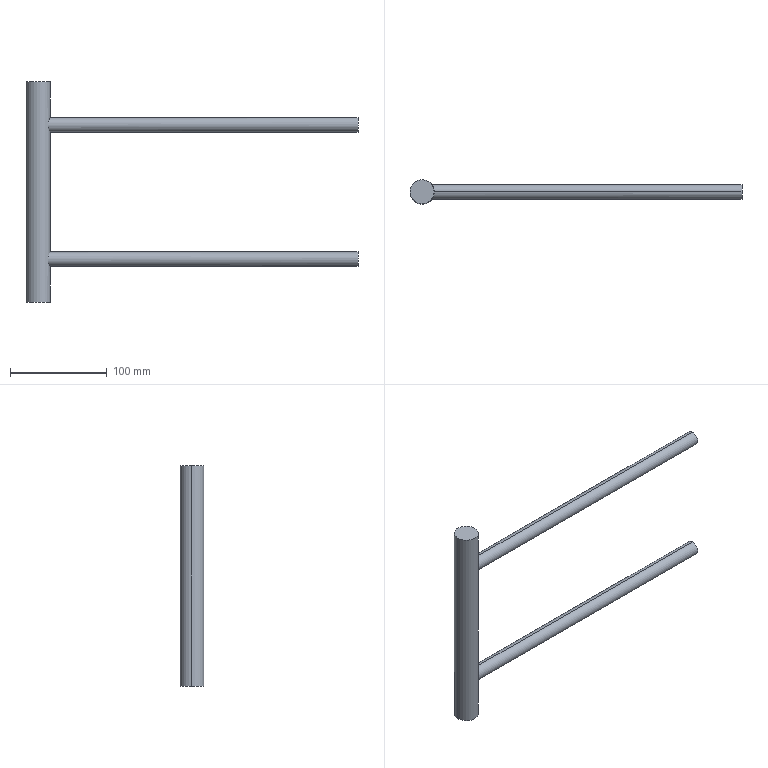Part | STEP file | Rear_Bar | 1 solid | 10 faces | box 343.5 x 25 x 228.558 mm | volume 224969 mm3 | cylinder 6 | plane 4 | commonest cylinder face diameters 15 x4 25 x2